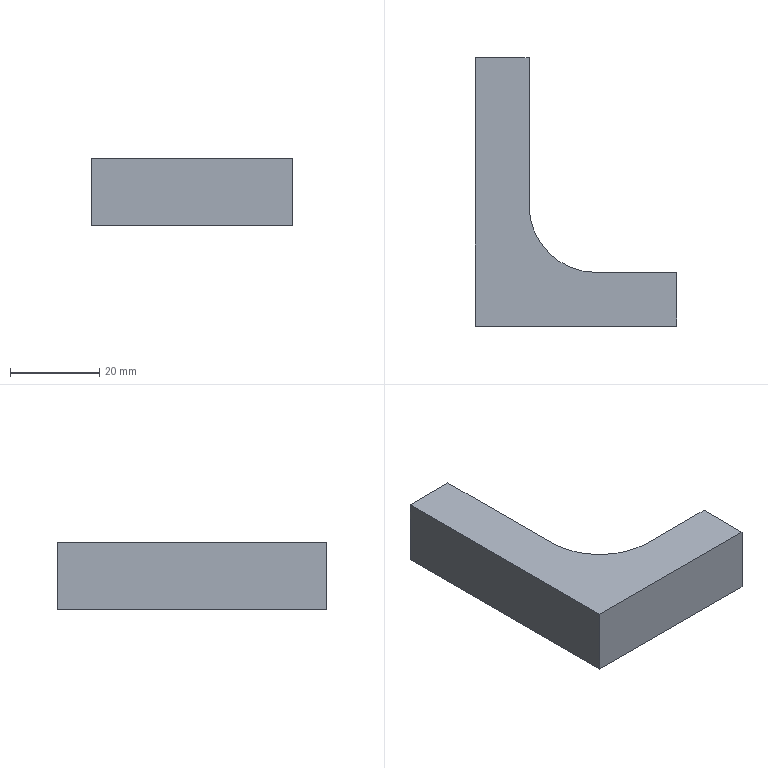Part | STEP file | 001-008-Traverse module reinforcing rib | 1 solid | 9 faces | box 45 x 60 x 15 mm | volume 17464 mm3 | plane 8 | cylinder 1 | commonest cylinder face diameters 30 x1
STEP:
#1=CARTESIAN_POINT('',(0.,0.,0.));
#2=DIRECTION('',(0.,0.,1.));
#3=DIRECTION('',(1.,0.,0.));
#4=AXIS2_PLACEMENT_3D('',#1,#2,#3);
#5=CARTESIAN_POINT('',(22.5,-30.,0.));
#6=VERTEX_POINT('',#5);
#7=CARTESIAN_POINT('',(22.5,-18.,0.));
#8=VERTEX_POINT('',#7);
#9=CARTESIAN_POINT('',(22.5,-30.,0.));
#10=DIRECTION('',(0.,1.,0.));
#11=VECTOR('',#10,1.);
#12=LINE('',#9,#11);
#13=CARTESIAN_POINT('',(22.5,-30.,15.));
#14=DIRECTION('',(-1.,0.,0.));
#15=DIRECTION('',(0.,-1.,0.));
#16=AXIS2_PLACEMENT_3D('',#13,#14,#15);
#17=PLANE('',#16);
#18=CARTESIAN_POINT('',(0.,-15.));
#19=DIRECTION('',(-1.,0.));
#20=VECTOR('',#19,1.);
#21=LINE('',#18,#20);
#22=(GEOMETRIC_REPRESENTATION_CONTEXT(2)PARAMETRIC_REPRESENTATION_CONTEXT()REPRESENTATION_CONTEXT('',''));
#23=DEFINITIONAL_REPRESENTATION('',(#21),#22);
#24=PCURVE('',#17,#23);
#25=CARTESIAN_POINT('',(0.,0.,0.));
#26=DIRECTION('',(0.,0.,-1.));
#27=DIRECTION('',(-1.,0.,0.));
#28=AXIS2_PLACEMENT_3D('',#25,#26,#27);
#29=PLANE('',#28);
#30=CARTESIAN_POINT('',(-22.5,-30.));
#31=DIRECTION('',(0.,1.));
#32=VECTOR('',#31,1.);
#33=LINE('',#30,#32);
#34=(GEOMETRIC_REPRESENTATION_CONTEXT(2)PARAMETRIC_REPRESENTATION_CONTEXT()REPRESENTATION_CONTEXT('',''));
#35=DEFINITIONAL_REPRESENTATION('',(#33),#34);
#36=PCURVE('',#29,#35);
#37=SURFACE_CURVE('',#12,(#24,#36),.PCURVE_S1.);
#38=EDGE_CURVE('',#6,#8,#37,.T.);
#39=ORIENTED_EDGE('',*,*,#38,.T.);
#40=CARTESIAN_POINT('',(22.5,-18.,15.));
#41=VERTEX_POINT('',#40);
#42=CARTESIAN_POINT('',(22.5,-18.,0.));
#43=DIRECTION('',(0.,0.,1.));
#44=VECTOR('',#43,1.);
#45=LINE('',#42,#44);
#46=CARTESIAN_POINT('',(-12.,-15.));
#47=DIRECTION('',(0.,1.));
#48=VECTOR('',#47,1.);
#49=LINE('',#46,#48);
#50=(GEOMETRIC_REPRESENTATION_CONTEXT(2)PARAMETRIC_REPRESENTATION_CONTEXT()REPRESENTATION_CONTEXT('',''));
#51=DEFINITIONAL_REPRESENTATION('',(#49),#50);
#52=PCURVE('',#17,#51);
#53=CARTESIAN_POINT('',(22.5,-18.,0.));
#54=DIRECTION('',(0.,-1.,0.));
#55=DIRECTION('',(0.,0.,-1.));
#56=AXIS2_PLACEMENT_3D('',#53,#54,#55);
#57=PLANE('',#56);
#58=CARTESIAN_POINT('',(0.,0.));
#59=DIRECTION('',(-1.,0.));
#60=VECTOR('',#59,1.);
#61=LINE('',#58,#60);
#62=(GEOMETRIC_REPRESENTATION_CONTEXT(2)PARAMETRIC_REPRESENTATION_CONTEXT()REPRESENTATION_CONTEXT('',''));
#63=DEFINITIONAL_REPRESENTATION('',(#61),#62);
#64=PCURVE('',#57,#63);
#65=SURFACE_CURVE('',#45,(#52,#64),.PCURVE_S1.);
#66=EDGE_CURVE('',#8,#41,#65,.T.);
#67=ORIENTED_EDGE('',*,*,#66,.T.);
#68=CARTESIAN_POINT('',(22.5,-30.,15.));
#69=VERTEX_POINT('',#68);
#70=CARTESIAN_POINT('',(22.5,-30.,15.));
#71=DIRECTION('',(0.,1.,0.));
#72=VECTOR('',#71,1.);
#73=LINE('',#70,#72);
#74=CARTESIAN_POINT('',(0.,0.));
#75=DIRECTION('',(-1.,0.));
#76=VECTOR('',#75,1.);
#77=LINE('',#74,#76);
#78=(GEOMETRIC_REPRESENTATION_CONTEXT(2)PARAMETRIC_REPRESENTATION_CONTEXT()REPRESENTATION_CONTEXT('',''));
#79=DEFINITIONAL_REPRESENTATION('',(#77),#78);
#80=PCURVE('',#17,#79);
#81=CARTESIAN_POINT('',(0.,0.,15.));
#82=DIRECTION('',(0.,0.,-1.));
#83=DIRECTION('',(-1.,0.,0.));
#84=AXIS2_PLACEMENT_3D('',#81,#82,#83);
#85=PLANE('',#84);
#86=CARTESIAN_POINT('',(-22.5,-30.));
#87=DIRECTION('',(0.,1.));
#88=VECTOR('',#87,1.);
#89=LINE('',#86,#88);
#90=(GEOMETRIC_REPRESENTATION_CONTEXT(2)PARAMETRIC_REPRESENTATION_CONTEXT()REPRESENTATION_CONTEXT('',''));
#91=DEFINITIONAL_REPRESENTATION('',(#89),#90);
#92=PCURVE('',#85,#91);
#93=SURFACE_CURVE('',#73,(#80,#92),.PCURVE_S1.);
#94=EDGE_CURVE('',#69,#41,#93,.T.);
#95=ORIENTED_EDGE('',*,*,#94,.F.);
#96=CARTESIAN_POINT('',(22.5,-30.,15.));
#97=DIRECTION('',(0.,0.,-1.));
#98=VECTOR('',#97,1.);
#99=LINE('',#96,#98);
#100=CARTESIAN_POINT('',(0.,0.));
#101=DIRECTION('',(0.,-1.));
#102=VECTOR('',#101,1.);
#103=LINE('',#100,#102);
#104=(GEOMETRIC_REPRESENTATION_CONTEXT(2)PARAMETRIC_REPRESENTATION_CONTEXT()REPRESENTATION_CONTEXT('',''));
#105=DEFINITIONAL_REPRESENTATION('',(#103),#104);
#106=PCURVE('',#17,#105);
#107=CARTESIAN_POINT('',(-22.5,-30.,15.));
#108=DIRECTION('',(0.,1.,0.));
#109=DIRECTION('',(-1.,0.,0.));
#110=AXIS2_PLACEMENT_3D('',#107,#108,#109);
#111=PLANE('',#110);
#112=CARTESIAN_POINT('',(-45.,0.));
#113=DIRECTION('',(0.,-1.));
#114=VECTOR('',#113,1.);
#115=LINE('',#112,#114);
#116=(GEOMETRIC_REPRESENTATION_CONTEXT(2)PARAMETRIC_REPRESENTATION_CONTEXT()REPRESENTATION_CONTEXT('',''));
#117=DEFINITIONAL_REPRESENTATION('',(#115),#116);
#118=PCURVE('',#111,#117);
#119=SURFACE_CURVE('',#99,(#106,#118),.PCURVE_S1.);
#120=EDGE_CURVE('',#69,#6,#119,.T.);
#121=ORIENTED_EDGE('',*,*,#120,.T.);
#122=EDGE_LOOP('',(#39,#67,#95,#121));
#123=FACE_BOUND('',#122,.T.);
#124=ADVANCED_FACE('',(#123),#17,.F.);
#125=CARTESIAN_POINT('',(-10.5,30.,15.));
#126=VERTEX_POINT('',#125);
#127=CARTESIAN_POINT('',(-22.5,30.,15.));
#128=VERTEX_POINT('',#127);
#129=CARTESIAN_POINT('',(-22.5,30.,15.));
#130=DIRECTION('',(-1.,0.,0.));
#131=VECTOR('',#130,1.);
#132=LINE('',#129,#131);
#133=CARTESIAN_POINT('',(-22.5,30.,15.));
#134=DIRECTION('',(0.,-1.,0.));
#135=DIRECTION('',(0.,0.,-1.));
#136=AXIS2_PLACEMENT_3D('',#133,#134,#135);
#137=PLANE('',#136);
#138=CARTESIAN_POINT('',(0.,0.));
#139=DIRECTION('',(0.,-1.));
#140=VECTOR('',#139,1.);
#141=LINE('',#138,#140);
#142=(GEOMETRIC_REPRESENTATION_CONTEXT(2)PARAMETRIC_REPRESENTATION_CONTEXT()REPRESENTATION_CONTEXT('',''));
#143=DEFINITIONAL_REPRESENTATION('',(#141),#142);
#144=PCURVE('',#137,#143);
#145=CARTESIAN_POINT('',(22.5,30.));
#146=DIRECTION('',(1.,0.));
#147=VECTOR('',#146,1.);
#148=LINE('',#145,#147);
#149=(GEOMETRIC_REPRESENTATION_CONTEXT(2)PARAMETRIC_REPRESENTATION_CONTEXT()REPRESENTATION_CONTEXT('',''));
#150=DEFINITIONAL_REPRESENTATION('',(#148),#149);
#151=PCURVE('',#85,#150);
#152=SURFACE_CURVE('',#132,(#144,#151),.PCURVE_S1.);
#153=EDGE_CURVE('',#126,#128,#152,.T.);
#154=ORIENTED_EDGE('',*,*,#153,.F.);
#155=CARTESIAN_POINT('',(-10.5,30.,0.));
#156=VERTEX_POINT('',#155);
#157=CARTESIAN_POINT('',(-10.5,30.,0.));
#158=DIRECTION('',(0.,0.,1.));
#159=VECTOR('',#158,1.);
#160=LINE('',#157,#159);
#161=CARTESIAN_POINT('',(15.,12.));
#162=DIRECTION('',(-1.,0.));
#163=VECTOR('',#162,1.);
#164=LINE('',#161,#163);
#165=(GEOMETRIC_REPRESENTATION_CONTEXT(2)PARAMETRIC_REPRESENTATION_CONTEXT()REPRESENTATION_CONTEXT('',''));
#166=DEFINITIONAL_REPRESENTATION('',(#164),#165);
#167=PCURVE('',#137,#166);
#168=CARTESIAN_POINT('',(-10.5,30.,0.));
#169=DIRECTION('',(-1.,0.,0.));
#170=DIRECTION('',(0.,0.,1.));
#171=AXIS2_PLACEMENT_3D('',#168,#169,#170);
#172=PLANE('',#171);
#173=CARTESIAN_POINT('',(0.,0.));
#174=DIRECTION('',(1.,0.));
#175=VECTOR('',#174,1.);
#176=LINE('',#173,#175);
#177=(GEOMETRIC_REPRESENTATION_CONTEXT(2)PARAMETRIC_REPRESENTATION_CONTEXT()REPRESENTATION_CONTEXT('',''));
#178=DEFINITIONAL_REPRESENTATION('',(#176),#177);
#179=PCURVE('',#172,#178);
#180=SURFACE_CURVE('',#160,(#167,#179),.PCURVE_S1.);
#181=EDGE_CURVE('',#156,#126,#180,.T.);
#182=ORIENTED_EDGE('',*,*,#181,.F.);
#183=CARTESIAN_POINT('',(-22.5,30.,0.));
#184=VERTEX_POINT('',#183);
#185=CARTESIAN_POINT('',(-22.5,30.,0.));
#186=DIRECTION('',(-1.,0.,0.));
#187=VECTOR('',#186,1.);
#188=LINE('',#185,#187);
#189=CARTESIAN_POINT('',(15.,0.));
#190=DIRECTION('',(0.,-1.));
#191=VECTOR('',#190,1.);
#192=LINE('',#189,#191);
#193=(GEOMETRIC_REPRESENTATION_CONTEXT(2)PARAMETRIC_REPRESENTATION_CONTEXT()REPRESENTATION_CONTEXT('',''));
#194=DEFINITIONAL_REPRESENTATION('',(#192),#193);
#195=PCURVE('',#137,#194);
#196=CARTESIAN_POINT('',(22.5,30.));
#197=DIRECTION('',(1.,0.));
#198=VECTOR('',#197,1.);
#199=LINE('',#196,#198);
#200=(GEOMETRIC_REPRESENTATION_CONTEXT(2)PARAMETRIC_REPRESENTATION_CONTEXT()REPRESENTATION_CONTEXT('',''));
#201=DEFINITIONAL_REPRESENTATION('',(#199),#200);
#202=PCURVE('',#29,#201);
#203=SURFACE_CURVE('',#188,(#195,#202),.PCURVE_S1.);
#204=EDGE_CURVE('',#156,#184,#203,.T.);
#205=ORIENTED_EDGE('',*,*,#204,.T.);
#206=CARTESIAN_POINT('',(-22.5,30.,15.));
#207=DIRECTION('',(0.,0.,-1.));
#208=VECTOR('',#207,1.);
#209=LINE('',#206,#208);
#210=CARTESIAN_POINT('',(0.,0.));
#211=DIRECTION('',(1.,0.));
#212=VECTOR('',#211,1.);
#213=LINE('',#210,#212);
#214=(GEOMETRIC_REPRESENTATION_CONTEXT(2)PARAMETRIC_REPRESENTATION_CONTEXT()REPRESENTATION_CONTEXT('',''));
#215=DEFINITIONAL_REPRESENTATION('',(#213),#214);
#216=PCURVE('',#137,#215);
#217=CARTESIAN_POINT('',(-22.5,-30.,15.));
#218=DIRECTION('',(1.,0.,0.));
#219=DIRECTION('',(0.,0.,-1.));
#220=AXIS2_PLACEMENT_3D('',#217,#218,#219);
#221=PLANE('',#220);
#222=CARTESIAN_POINT('',(0.,60.));
#223=DIRECTION('',(1.,0.));
#224=VECTOR('',#223,1.);
#225=LINE('',#222,#224);
#226=(GEOMETRIC_REPRESENTATION_CONTEXT(2)PARAMETRIC_REPRESENTATION_CONTEXT()REPRESENTATION_CONTEXT('',''));
#227=DEFINITIONAL_REPRESENTATION('',(#225),#226);
#228=PCURVE('',#221,#227);
#229=SURFACE_CURVE('',#209,(#216,#228),.PCURVE_S1.);
#230=EDGE_CURVE('',#128,#184,#229,.T.);
#231=ORIENTED_EDGE('',*,*,#230,.F.);
#232=EDGE_LOOP('',(#154,#182,#205,#231));
#233=FACE_BOUND('',#232,.T.);
#234=ADVANCED_FACE('',(#233),#137,.F.);
#235=CARTESIAN_POINT('',(-22.5,-30.,0.));
#236=VERTEX_POINT('',#235);
#237=CARTESIAN_POINT('',(-22.5,-30.,0.));
#238=DIRECTION('',(0.,-1.,0.));
#239=VECTOR('',#238,1.);
#240=LINE('',#237,#239);
#241=CARTESIAN_POINT('',(15.,0.));
#242=DIRECTION('',(0.,-1.));
#243=VECTOR('',#242,1.);
#244=LINE('',#241,#243);
#245=(GEOMETRIC_REPRESENTATION_CONTEXT(2)PARAMETRIC_REPRESENTATION_CONTEXT()REPRESENTATION_CONTEXT('',''));
#246=DEFINITIONAL_REPRESENTATION('',(#244),#245);
#247=PCURVE('',#221,#246);
#248=CARTESIAN_POINT('',(22.5,-30.));
#249=DIRECTION('',(0.,-1.));
#250=VECTOR('',#249,1.);
#251=LINE('',#248,#250);
#252=(GEOMETRIC_REPRESENTATION_CONTEXT(2)PARAMETRIC_REPRESENTATION_CONTEXT()REPRESENTATION_CONTEXT('',''));
#253=DEFINITIONAL_REPRESENTATION('',(#251),#252);
#254=PCURVE('',#29,#253);
#255=SURFACE_CURVE('',#240,(#247,#254),.PCURVE_S1.);
#256=EDGE_CURVE('',#184,#236,#255,.T.);
#257=ORIENTED_EDGE('',*,*,#256,.T.);
#258=CARTESIAN_POINT('',(-22.5,-30.,15.));
#259=VERTEX_POINT('',#258);
#260=CARTESIAN_POINT('',(-22.5,-30.,15.));
#261=DIRECTION('',(0.,0.,-1.));
#262=VECTOR('',#261,1.);
#263=LINE('',#260,#262);
#264=CARTESIAN_POINT('',(0.,0.));
#265=DIRECTION('',(1.,0.));
#266=VECTOR('',#265,1.);
#267=LINE('',#264,#266);
#268=(GEOMETRIC_REPRESENTATION_CONTEXT(2)PARAMETRIC_REPRESENTATION_CONTEXT()REPRESENTATION_CONTEXT('',''));
#269=DEFINITIONAL_REPRESENTATION('',(#267),#268);
#270=PCURVE('',#221,#269);
#271=CARTESIAN_POINT('',(0.,0.));
#272=DIRECTION('',(0.,-1.));
#273=VECTOR('',#272,1.);
#274=LINE('',#271,#273);
#275=(GEOMETRIC_REPRESENTATION_CONTEXT(2)PARAMETRIC_REPRESENTATION_CONTEXT()REPRESENTATION_CONTEXT('',''));
#276=DEFINITIONAL_REPRESENTATION('',(#274),#275);
#277=PCURVE('',#111,#276);
#278=SURFACE_CURVE('',#263,(#270,#277),.PCURVE_S1.);
#279=EDGE_CURVE('',#259,#236,#278,.T.);
#280=ORIENTED_EDGE('',*,*,#279,.F.);
#281=CARTESIAN_POINT('',(-22.5,-30.,15.));
#282=DIRECTION('',(0.,-1.,0.));
#283=VECTOR('',#282,1.);
#284=LINE('',#281,#283);
#285=CARTESIAN_POINT('',(0.,0.));
#286=DIRECTION('',(0.,-1.));
#287=VECTOR('',#286,1.);
#288=LINE('',#285,#287);
#289=(GEOMETRIC_REPRESENTATION_CONTEXT(2)PARAMETRIC_REPRESENTATION_CONTEXT()REPRESENTATION_CONTEXT('',''));
#290=DEFINITIONAL_REPRESENTATION('',(#288),#289);
#291=PCURVE('',#221,#290);
#292=CARTESIAN_POINT('',(22.5,-30.));
#293=DIRECTION('',(0.,-1.));
#294=VECTOR('',#293,1.);
#295=LINE('',#292,#294);
#296=(GEOMETRIC_REPRESENTATION_CONTEXT(2)PARAMETRIC_REPRESENTATION_CONTEXT()REPRESENTATION_CONTEXT('',''));
#297=DEFINITIONAL_REPRESENTATION('',(#295),#296);
#298=PCURVE('',#85,#297);
#299=SURFACE_CURVE('',#284,(#291,#298),.PCURVE_S1.);
#300=EDGE_CURVE('',#128,#259,#299,.T.);
#301=ORIENTED_EDGE('',*,*,#300,.F.);
#302=ORIENTED_EDGE('',*,*,#230,.T.);
#303=EDGE_LOOP('',(#257,#280,#301,#302));
#304=FACE_BOUND('',#303,.T.);
#305=ADVANCED_FACE('',(#304),#221,.F.);
#306=CARTESIAN_POINT('',(-22.5,-30.,0.));
#307=DIRECTION('',(1.,0.,0.));
#308=VECTOR('',#307,1.);
#309=LINE('',#306,#308);
#310=CARTESIAN_POINT('',(0.,-15.));
#311=DIRECTION('',(-1.,0.));
#312=VECTOR('',#311,1.);
#313=LINE('',#310,#312);
#314=(GEOMETRIC_REPRESENTATION_CONTEXT(2)PARAMETRIC_REPRESENTATION_CONTEXT()REPRESENTATION_CONTEXT('',''));
#315=DEFINITIONAL_REPRESENTATION('',(#313),#314);
#316=PCURVE('',#111,#315);
#317=CARTESIAN_POINT('',(22.5,-30.));
#318=DIRECTION('',(-1.,0.));
#319=VECTOR('',#318,1.);
#320=LINE('',#317,#319);
#321=(GEOMETRIC_REPRESENTATION_CONTEXT(2)PARAMETRIC_REPRESENTATION_CONTEXT()REPRESENTATION_CONTEXT('',''));
#322=DEFINITIONAL_REPRESENTATION('',(#320),#321);
#323=PCURVE('',#29,#322);
#324=SURFACE_CURVE('',#309,(#316,#323),.PCURVE_S1.);
#325=EDGE_CURVE('',#236,#6,#324,.T.);
#326=ORIENTED_EDGE('',*,*,#325,.T.);
#327=ORIENTED_EDGE('',*,*,#120,.F.);
#328=CARTESIAN_POINT('',(-22.5,-30.,15.));
#329=DIRECTION('',(1.,0.,0.));
#330=VECTOR('',#329,1.);
#331=LINE('',#328,#330);
#332=CARTESIAN_POINT('',(0.,0.));
#333=DIRECTION('',(-1.,0.));
#334=VECTOR('',#333,1.);
#335=LINE('',#332,#334);
#336=(GEOMETRIC_REPRESENTATION_CONTEXT(2)PARAMETRIC_REPRESENTATION_CONTEXT()REPRESENTATION_CONTEXT('',''));
#337=DEFINITIONAL_REPRESENTATION('',(#335),#336);
#338=PCURVE('',#111,#337);
#339=CARTESIAN_POINT('',(22.5,-30.));
#340=DIRECTION('',(-1.,0.));
#341=VECTOR('',#340,1.);
#342=LINE('',#339,#341);
#343=(GEOMETRIC_REPRESENTATION_CONTEXT(2)PARAMETRIC_REPRESENTATION_CONTEXT()REPRESENTATION_CONTEXT('',''));
#344=DEFINITIONAL_REPRESENTATION('',(#342),#343);
#345=PCURVE('',#85,#344);
#346=SURFACE_CURVE('',#331,(#338,#345),.PCURVE_S1.);
#347=EDGE_CURVE('',#259,#69,#346,.T.);
#348=ORIENTED_EDGE('',*,*,#347,.F.);
#349=ORIENTED_EDGE('',*,*,#279,.T.);
#350=EDGE_LOOP('',(#326,#327,#348,#349));
#351=FACE_BOUND('',#350,.T.);
#352=ADVANCED_FACE('',(#351),#111,.F.);
#353=ORIENTED_EDGE('',*,*,#94,.T.);
#354=CARTESIAN_POINT('',(4.5,-18.,15.));
#355=VERTEX_POINT('',#354);
#356=CARTESIAN_POINT('',(22.5,-18.,15.));
#357=DIRECTION('',(1.,0.,0.));
#358=VECTOR('',#357,1.);
#359=LINE('',#356,#358);
#360=CARTESIAN_POINT('',(-22.5,-18.));
#361=DIRECTION('',(-1.,0.));
#362=VECTOR('',#361,1.);
#363=LINE('',#360,#362);
#364=(GEOMETRIC_REPRESENTATION_CONTEXT(2)PARAMETRIC_REPRESENTATION_CONTEXT()REPRESENTATION_CONTEXT('',''));
#365=DEFINITIONAL_REPRESENTATION('',(#363),#364);
#366=PCURVE('',#85,#365);
#367=CARTESIAN_POINT('',(-15.,0.));
#368=DIRECTION('',(0.,1.));
#369=VECTOR('',#368,1.);
#370=LINE('',#367,#369);
#371=(GEOMETRIC_REPRESENTATION_CONTEXT(2)PARAMETRIC_REPRESENTATION_CONTEXT()REPRESENTATION_CONTEXT('',''));
#372=DEFINITIONAL_REPRESENTATION('',(#370),#371);
#373=PCURVE('',#57,#372);
#374=SURFACE_CURVE('',#359,(#366,#373),.PCURVE_S1.);
#375=EDGE_CURVE('',#355,#41,#374,.T.);
#376=ORIENTED_EDGE('',*,*,#375,.F.);
#377=CARTESIAN_POINT('',(-10.5,-3.,15.));
#378=VERTEX_POINT('',#377);
#379=CARTESIAN_POINT('',(4.5,-3.,15.));
#380=DIRECTION('',(0.,0.,-1.));
#381=DIRECTION('',(-1.,0.,0.));
#382=AXIS2_PLACEMENT_3D('',#379,#380,#381);
#383=CIRCLE('',#382,15.);
#384=CARTESIAN_POINT('',(-4.5,-3.));
#385=DIRECTION('',(1.,0.));
#386=AXIS2_PLACEMENT_2D('',#384,#385);
#387=CIRCLE('',#386,15.);
#388=(GEOMETRIC_REPRESENTATION_CONTEXT(2)PARAMETRIC_REPRESENTATION_CONTEXT()REPRESENTATION_CONTEXT('',''));
#389=DEFINITIONAL_REPRESENTATION('',(#387),#388);
#390=PCURVE('',#85,#389);
#391=CARTESIAN_POINT('',(4.5,-3.,0.));
#392=DIRECTION('',(0.,0.,-1.));
#393=DIRECTION('',(-1.,0.,0.));
#394=AXIS2_PLACEMENT_3D('',#391,#392,#393);
#395=CYLINDRICAL_SURFACE('',#394,15.);
#396=CARTESIAN_POINT('',(0.,-15.));
#397=DIRECTION('',(1.,0.));
#398=VECTOR('',#397,1.);
#399=LINE('',#396,#398);
#400=(GEOMETRIC_REPRESENTATION_CONTEXT(2)PARAMETRIC_REPRESENTATION_CONTEXT()REPRESENTATION_CONTEXT('',''));
#401=DEFINITIONAL_REPRESENTATION('',(#399),#400);
#402=PCURVE('',#395,#401);
#403=SURFACE_CURVE('',#383,(#390,#402),.PCURVE_S1.);
#404=EDGE_CURVE('',#355,#378,#403,.T.);
#405=ORIENTED_EDGE('',*,*,#404,.T.);
#406=CARTESIAN_POINT('',(-10.5,30.,15.));
#407=DIRECTION('',(0.,-1.,0.));
#408=VECTOR('',#407,1.);
#409=LINE('',#406,#408);
#410=CARTESIAN_POINT('',(10.5,30.));
#411=DIRECTION('',(0.,-1.));
#412=VECTOR('',#411,1.);
#413=LINE('',#410,#412);
#414=(GEOMETRIC_REPRESENTATION_CONTEXT(2)PARAMETRIC_REPRESENTATION_CONTEXT()REPRESENTATION_CONTEXT('',''));
#415=DEFINITIONAL_REPRESENTATION('',(#413),#414);
#416=PCURVE('',#85,#415);
#417=CARTESIAN_POINT('',(15.,0.));
#418=DIRECTION('',(0.,-1.));
#419=VECTOR('',#418,1.);
#420=LINE('',#417,#419);
#421=(GEOMETRIC_REPRESENTATION_CONTEXT(2)PARAMETRIC_REPRESENTATION_CONTEXT()REPRESENTATION_CONTEXT('',''));
#422=DEFINITIONAL_REPRESENTATION('',(#420),#421);
#423=PCURVE('',#172,#422);
#424=SURFACE_CURVE('',#409,(#416,#423),.PCURVE_S1.);
#425=EDGE_CURVE('',#126,#378,#424,.T.);
#426=ORIENTED_EDGE('',*,*,#425,.F.);
#427=ORIENTED_EDGE('',*,*,#153,.T.);
#428=ORIENTED_EDGE('',*,*,#300,.T.);
#429=ORIENTED_EDGE('',*,*,#347,.T.);
#430=EDGE_LOOP('',(#353,#376,#405,#426,#427,#428,#429));
#431=FACE_BOUND('',#430,.T.);
#432=ADVANCED_FACE('',(#431),#85,.F.);
#433=CARTESIAN_POINT('',(-10.5,-3.,0.));
#434=VERTEX_POINT('',#433);
#435=CARTESIAN_POINT('',(-10.5,30.,0.));
#436=DIRECTION('',(0.,-1.,0.));
#437=VECTOR('',#436,1.);
#438=LINE('',#435,#437);
#439=CARTESIAN_POINT('',(10.5,30.));
#440=DIRECTION('',(0.,-1.));
#441=VECTOR('',#440,1.);
#442=LINE('',#439,#441);
#443=(GEOMETRIC_REPRESENTATION_CONTEXT(2)PARAMETRIC_REPRESENTATION_CONTEXT()REPRESENTATION_CONTEXT('',''));
#444=DEFINITIONAL_REPRESENTATION('',(#442),#443);
#445=PCURVE('',#29,#444);
#446=CARTESIAN_POINT('',(0.,0.));
#447=DIRECTION('',(0.,-1.));
#448=VECTOR('',#447,1.);
#449=LINE('',#446,#448);
#450=(GEOMETRIC_REPRESENTATION_CONTEXT(2)PARAMETRIC_REPRESENTATION_CONTEXT()REPRESENTATION_CONTEXT('',''));
#451=DEFINITIONAL_REPRESENTATION('',(#449),#450);
#452=PCURVE('',#172,#451);
#453=SURFACE_CURVE('',#438,(#445,#452),.PCURVE_S1.);
#454=EDGE_CURVE('',#156,#434,#453,.T.);
#455=ORIENTED_EDGE('',*,*,#454,.T.);
#456=CARTESIAN_POINT('',(4.5,-18.,0.));
#457=VERTEX_POINT('',#456);
#458=CARTESIAN_POINT('',(4.5,-3.,0.));
#459=DIRECTION('',(0.,0.,1.));
#460=DIRECTION('',(-1.,0.,0.));
#461=AXIS2_PLACEMENT_3D('',#458,#459,#460);
#462=CIRCLE('',#461,15.);
#463=CARTESIAN_POINT('',(10.5,-3.));
#464=CARTESIAN_POINT('',(10.5,-28.981));
#465=CARTESIAN_POINT('',(-12.,-15.99));
#466=CARTESIAN_POINT('',(-34.5,-3.));
#467=CARTESIAN_POINT('',(-12.,9.99));
#468=CARTESIAN_POINT('',(10.5,22.981));
#469=CARTESIAN_POINT('',(10.5,-3.));
#470=(BOUNDED_CURVE()B_SPLINE_CURVE(2,(#463,#464,#465,#466,#467,#468,#469),.UNSPECIFIED.,.T.,.F.)B_SPLINE_CURVE_WITH_KNOTS((1,2,2,2,2,1),(-2.094,0.,2.094,4.189,6.283,8.378),.UNSPECIFIED.)CURVE()GEOMETRIC_REPRESENTATION_ITEM()RATIONAL_B_SPLINE_CURVE((1.,0.5,1.,0.5,1.,0.5,1.))REPRESENTATION_ITEM(''));
#471=(GEOMETRIC_REPRESENTATION_CONTEXT(2)PARAMETRIC_REPRESENTATION_CONTEXT()REPRESENTATION_CONTEXT('',''));
#472=DEFINITIONAL_REPRESENTATION('',(#470),#471);
#473=PCURVE('',#29,#472);
#474=CARTESIAN_POINT('',(6.283,0.));
#475=DIRECTION('',(-1.,0.));
#476=VECTOR('',#475,1.);
#477=LINE('',#474,#476);
#478=(GEOMETRIC_REPRESENTATION_CONTEXT(2)PARAMETRIC_REPRESENTATION_CONTEXT()REPRESENTATION_CONTEXT('',''));
#479=DEFINITIONAL_REPRESENTATION('',(#477),#478);
#480=PCURVE('',#395,#479);
#481=SURFACE_CURVE('',#462,(#473,#480),.PCURVE_S1.);
#482=EDGE_CURVE('',#434,#457,#481,.T.);
#483=ORIENTED_EDGE('',*,*,#482,.T.);
#484=CARTESIAN_POINT('',(22.5,-18.,0.));
#485=DIRECTION('',(1.,0.,0.));
#486=VECTOR('',#485,1.);
#487=LINE('',#484,#486);
#488=CARTESIAN_POINT('',(-22.5,-18.));
#489=DIRECTION('',(-1.,0.));
#490=VECTOR('',#489,1.);
#491=LINE('',#488,#490);
#492=(GEOMETRIC_REPRESENTATION_CONTEXT(2)PARAMETRIC_REPRESENTATION_CONTEXT()REPRESENTATION_CONTEXT('',''));
#493=DEFINITIONAL_REPRESENTATION('',(#491),#492);
#494=PCURVE('',#29,#493);
#495=CARTESIAN_POINT('',(0.,0.));
#496=DIRECTION('',(0.,1.));
#497=VECTOR('',#496,1.);
#498=LINE('',#495,#497);
#499=(GEOMETRIC_REPRESENTATION_CONTEXT(2)PARAMETRIC_REPRESENTATION_CONTEXT()REPRESENTATION_CONTEXT('',''));
#500=DEFINITIONAL_REPRESENTATION('',(#498),#499);
#501=PCURVE('',#57,#500);
#502=SURFACE_CURVE('',#487,(#494,#501),.PCURVE_S1.);
#503=EDGE_CURVE('',#457,#8,#502,.T.);
#504=ORIENTED_EDGE('',*,*,#503,.T.);
#505=ORIENTED_EDGE('',*,*,#38,.F.);
#506=ORIENTED_EDGE('',*,*,#325,.F.);
#507=ORIENTED_EDGE('',*,*,#256,.F.);
#508=ORIENTED_EDGE('',*,*,#204,.F.);
#509=EDGE_LOOP('',(#455,#483,#504,#505,#506,#507,#508));
#510=FACE_BOUND('',#509,.T.);
#511=ADVANCED_FACE('',(#510),#29,.T.);
#512=ORIENTED_EDGE('',*,*,#503,.F.);
#513=CARTESIAN_POINT('',(4.5,-18.,15.));
#514=DIRECTION('',(0.,0.,1.));
#515=VECTOR('',#514,1.);
#516=LINE('',#513,#515);
#517=CARTESIAN_POINT('',(-15.,-18.));
#518=DIRECTION('',(-1.,0.));
#519=VECTOR('',#518,1.);
#520=LINE('',#517,#519);
#521=(GEOMETRIC_REPRESENTATION_CONTEXT(2)PARAMETRIC_REPRESENTATION_CONTEXT()REPRESENTATION_CONTEXT('',''));
#522=DEFINITIONAL_REPRESENTATION('',(#520),#521);
#523=PCURVE('',#57,#522);
#524=CARTESIAN_POINT('',(4.712,-15.));
#525=DIRECTION('',(0.,-1.));
#526=VECTOR('',#525,1.);
#527=LINE('',#524,#526);
#528=(GEOMETRIC_REPRESENTATION_CONTEXT(2)PARAMETRIC_REPRESENTATION_CONTEXT()REPRESENTATION_CONTEXT('',''));
#529=DEFINITIONAL_REPRESENTATION('',(#527),#528);
#530=PCURVE('',#395,#529);
#531=SURFACE_CURVE('',#516,(#523,#530),.PCURVE_S1.);
#532=EDGE_CURVE('',#457,#355,#531,.T.);
#533=ORIENTED_EDGE('',*,*,#532,.T.);
#534=ORIENTED_EDGE('',*,*,#375,.T.);
#535=ORIENTED_EDGE('',*,*,#66,.F.);
#536=EDGE_LOOP('',(#512,#533,#534,#535));
#537=FACE_BOUND('',#536,.T.);
#538=ADVANCED_FACE('',(#537),#57,.F.);
#539=ORIENTED_EDGE('',*,*,#425,.T.);
#540=CARTESIAN_POINT('',(-10.5,-3.,0.));
#541=DIRECTION('',(0.,0.,-1.));
#542=VECTOR('',#541,1.);
#543=LINE('',#540,#542);
#544=CARTESIAN_POINT('',(0.,-33.));
#545=DIRECTION('',(-1.,0.));
#546=VECTOR('',#545,1.);
#547=LINE('',#544,#546);
#548=(GEOMETRIC_REPRESENTATION_CONTEXT(2)PARAMETRIC_REPRESENTATION_CONTEXT()REPRESENTATION_CONTEXT('',''));
#549=DEFINITIONAL_REPRESENTATION('',(#547),#548);
#550=PCURVE('',#172,#549);
#551=CARTESIAN_POINT('',(6.283,0.));
#552=DIRECTION('',(0.,1.));
#553=VECTOR('',#552,1.);
#554=LINE('',#551,#553);
#555=(GEOMETRIC_REPRESENTATION_CONTEXT(2)PARAMETRIC_REPRESENTATION_CONTEXT()REPRESENTATION_CONTEXT('',''));
#556=DEFINITIONAL_REPRESENTATION('',(#554),#555);
#557=PCURVE('',#395,#556);
#558=SURFACE_CURVE('',#543,(#550,#557),.PCURVE_S1.);
#559=EDGE_CURVE('',#378,#434,#558,.T.);
#560=ORIENTED_EDGE('',*,*,#559,.T.);
#561=ORIENTED_EDGE('',*,*,#454,.F.);
#562=ORIENTED_EDGE('',*,*,#181,.T.);
#563=EDGE_LOOP('',(#539,#560,#561,#562));
#564=FACE_BOUND('',#563,.T.);
#565=ADVANCED_FACE('',(#564),#172,.F.);
#566=ORIENTED_EDGE('',*,*,#532,.T.);
#567=ORIENTED_EDGE('',*,*,#404,.T.);
#568=ORIENTED_EDGE('',*,*,#559,.T.);
#569=ORIENTED_EDGE('',*,*,#482,.T.);
#570=EDGE_LOOP('',(#566,#567,#568,#569));
#571=FACE_BOUND('',#570,.F.);
#572=ADVANCED_FACE('',(#571),#395,.F.);
#573=CLOSED_SHELL('',(#124,#234,#305,#352,#432,#511,#538,#565,#572));
#574=MANIFOLD_SOLID_BREP('',#573);
#575=(LENGTH_UNIT()NAMED_UNIT(*)SI_UNIT(.MILLI.,.METRE.));
#576=UNCERTAINTY_MEASURE_WITH_UNIT(LENGTH_MEASURE(0.0000001),#575,'','');
#577=(NAMED_UNIT(*)PLANE_ANGLE_UNIT()SI_UNIT($,.RADIAN.));
#578=(NAMED_UNIT(*)SI_UNIT($,.STERADIAN.)SOLID_ANGLE_UNIT());
#579=(GEOMETRIC_REPRESENTATION_CONTEXT(3)GLOBAL_UNCERTAINTY_ASSIGNED_CONTEXT((#576))GLOBAL_UNIT_ASSIGNED_CONTEXT((#575,#577,#578))REPRESENTATION_CONTEXT('',''));
#580=ADVANCED_BREP_SHAPE_REPRESENTATION('',(#4,#574),#579);